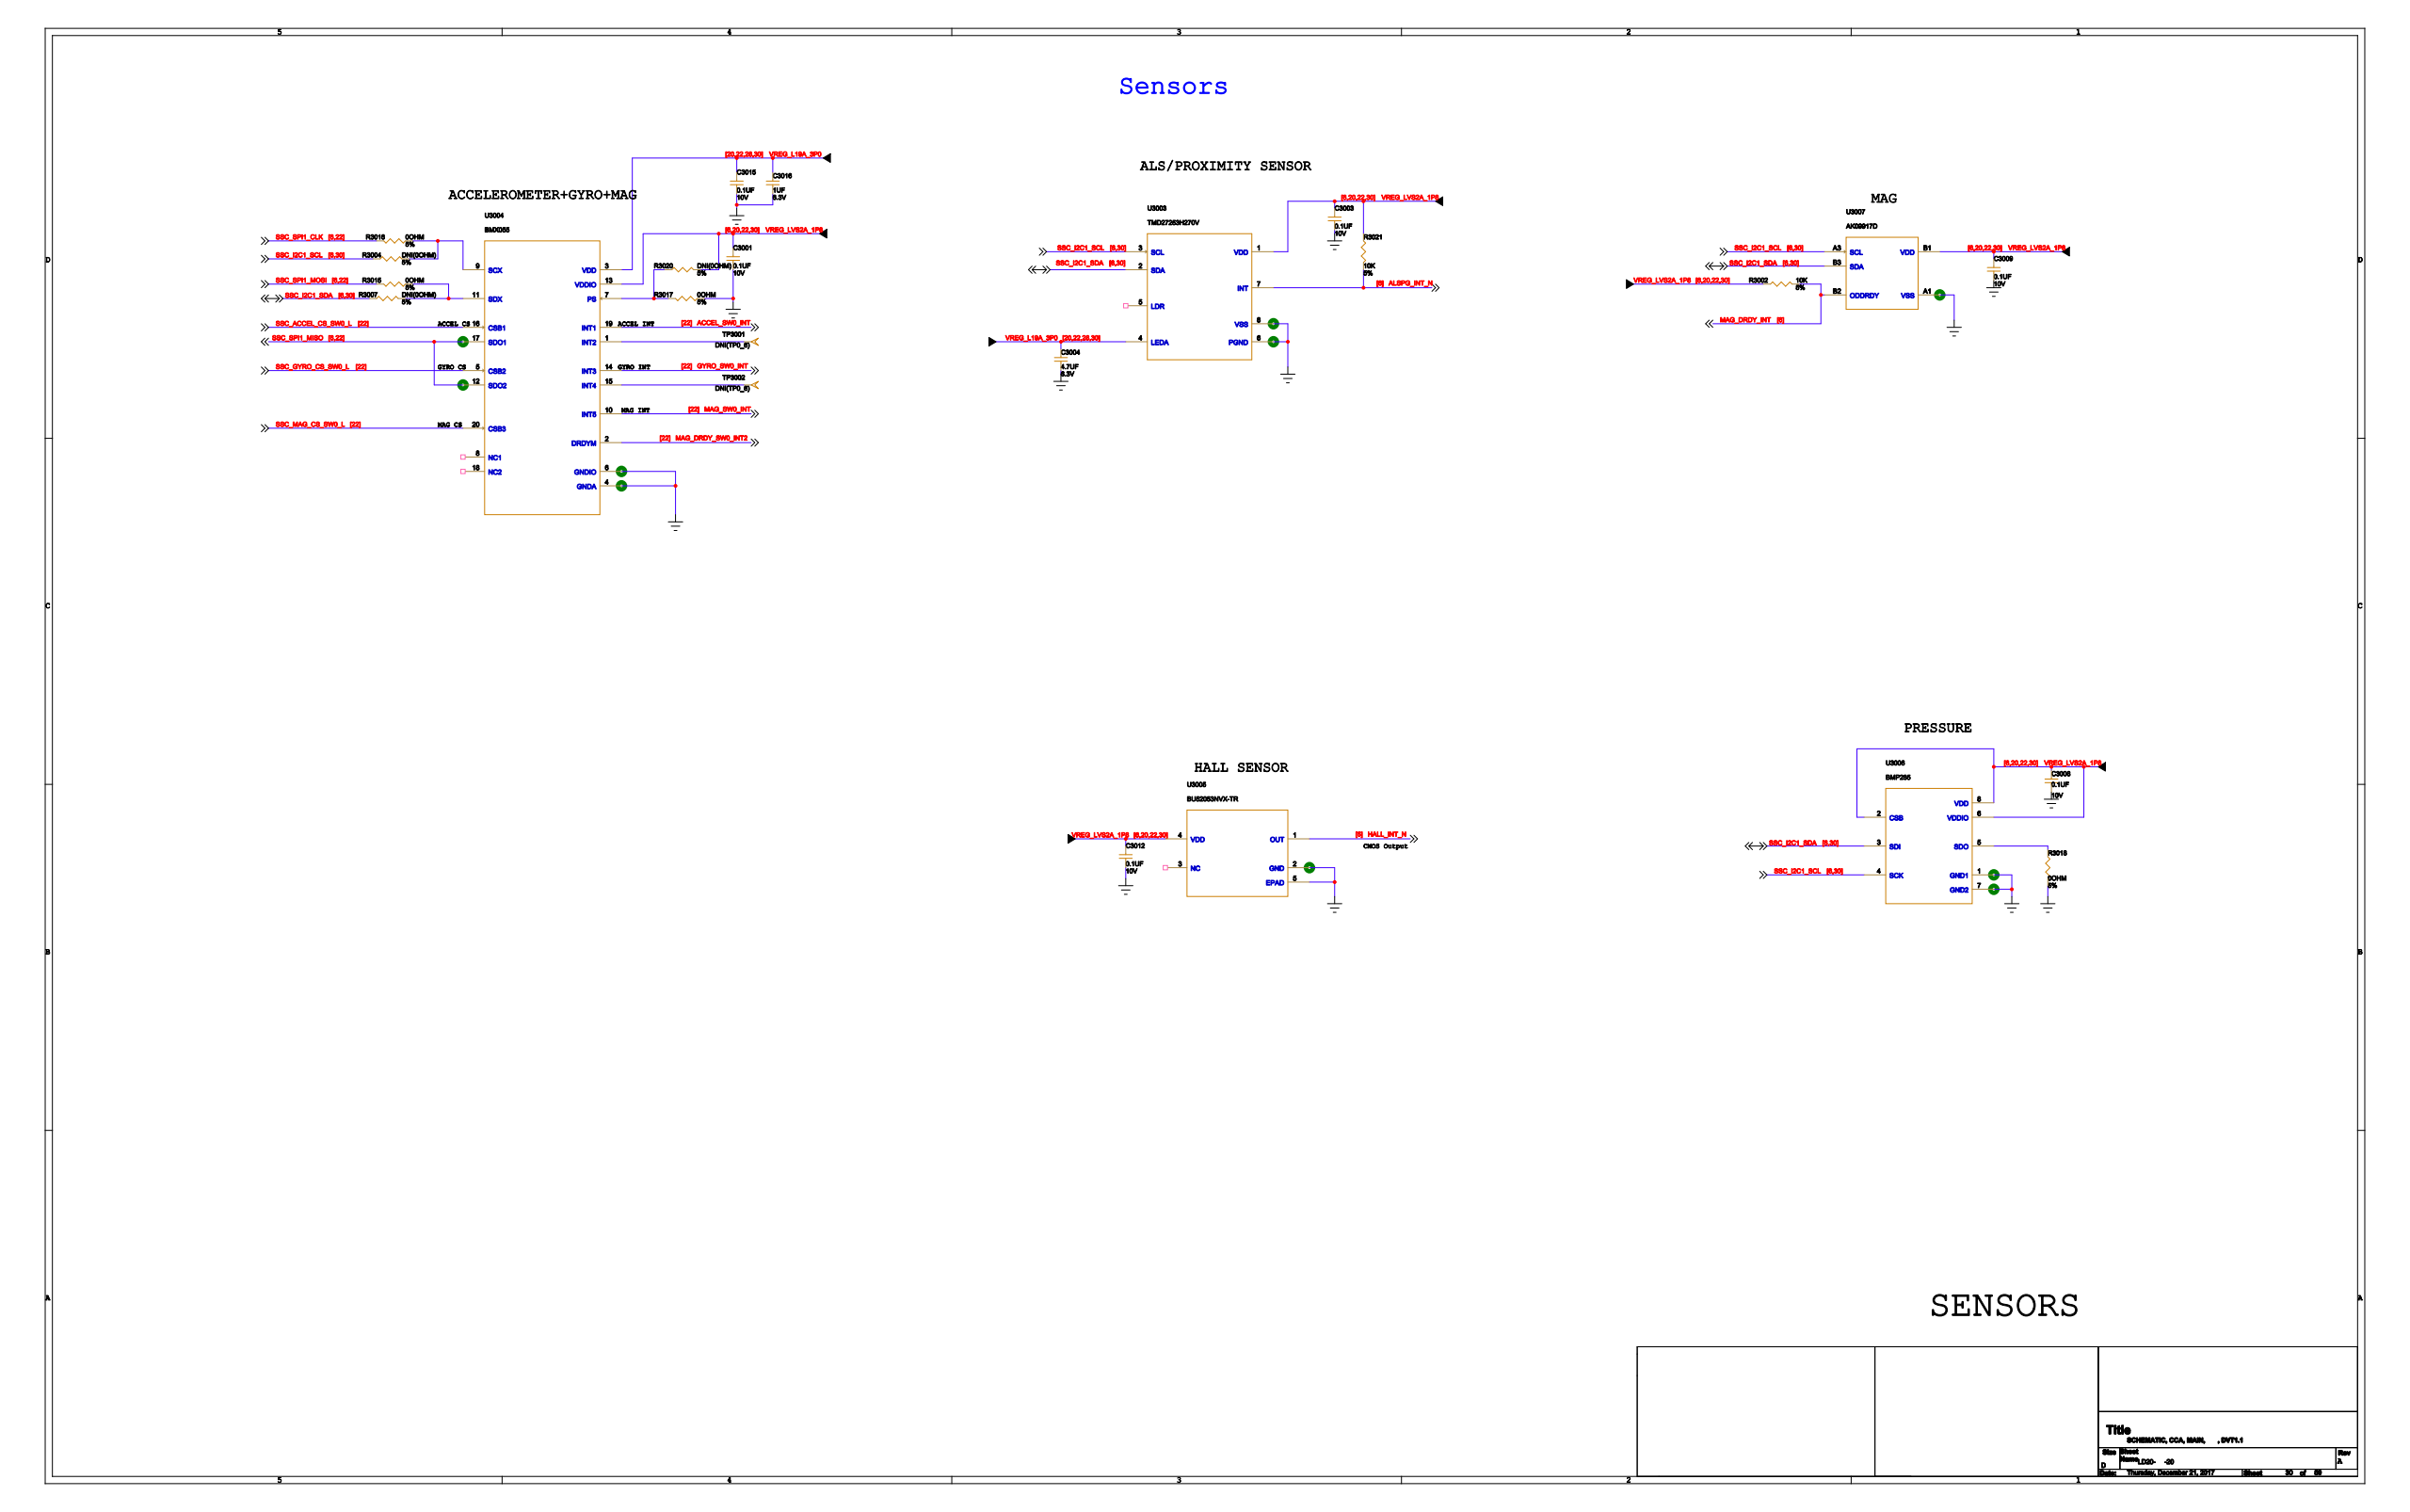Circuit board | Cadence Allegro | 1520 parts | 1149 nets | one sheet of the schematic
Parts on this sheet (reference | value | footprint):
C3001 | 0.1UF | 2P0201R
C3003 | 0.1UF | 2P0201R
C3004 | 4.7UF | 2P0402R
C3008 | 0.1UF | 2P0201R
C3009 | 0.1UF | 2P0201R
C3012 | 0.1UF | 2P0201R
C3015 | 0.1UF | 2P0201R
C3016 | 1UF | 2P0201R
R3002 | 10K | 2P0201R
R3004 | DNI(0OHM) | 2P0201R_DNI
R3007 | DNI(0OHM) | 2P0201R_DNI
R3015 | 0OHM | 2P0201R
R3016 | 0OHM | 2P0201R
R3017 | 0OHM | 2P0201R
R3018 | 0OHM | 2P0201R
R3020 | DNI(0OHM) | 2P0201R_DNI
R3021 | 10K | 2P0201R
TP3001 | DNI(TP0_6) | TP-0_6
TP3002 | DNI(TP0_6) | TP-0_6
U3003 | TMD27253H270V | 8PSM163X98N
U3004 | BMX055 | 20LGA181X122N197
U3005 | BU52053NVX-TR | 5PSM51X67N
U3006 | BMP285 | 8PSM102X83N256
U3007 | AK09917D | 5PGA32X48B157V1
Nets of these parts (net: part-pin ...):
GND: C3001-2 C3003-2 C3004-2 C3008-2 C3009-2 C3012-2 C3015-2 C3016-2 R3017-2 R3018-1 U3003-6 U3003-8 U3004-4 U3004-6 U3005-2 U3005-5 U3006-1 U3006-7 U3007-A1
ALSPG_INT_N: R3021-1 U3003-7
VREG_L19A_3P0: C3004-1 C3015-1 C3016-1 U3003-4 U3004-3
SSC_I2C1_SCL: R3004-2 U3003-3 U3006-4 U3007-A3
SSC_I2C1_SDA: R3007-2 U3003-2 U3006-3 U3007-B3
VREG_LVS2A_1P8: C3001-1 C3003-1 C3008-1 C3009-1 C3012-1 R3002-2 R3020-1 R3021-2 U3003-1 U3004-13 U3005-4 U3006-2 U3006-6 U3006-8 U3007-B1
SSC_SPI1_MISO: U3004-12 U3004-17
SSC_SPI1_MOSI: R3015-1
SSC_SPI1_CLK: R3016-1
SSC_MAG_CS_SW0_L: U3004-20
SSC_ACCEL_CS_SW0_L: U3004-16
SSC_GYRO_CS_SW0_L: U3004-5
MAG_SW0_INT: U3004-10
MAG_DRDY_SW0_INT2: U3004-2
ACCEL_SW0_INT: U3004-19
GYRO_SW0_INT: U3004-14
MAG_DRDY_INT: R3002-1 U3007-B2
N49627982: R3007-1 R3015-2 U3004-11
N49627992: R3004-1 R3016-2 U3004-9
N49628666: R3017-1 R3020-2 U3004-7
N34237798: R3018-2 U3006-5
N49470572: TP3001-1 U3004-1
N49470582: TP3002-1 U3004-15
HALL_INT_N: U3005-1